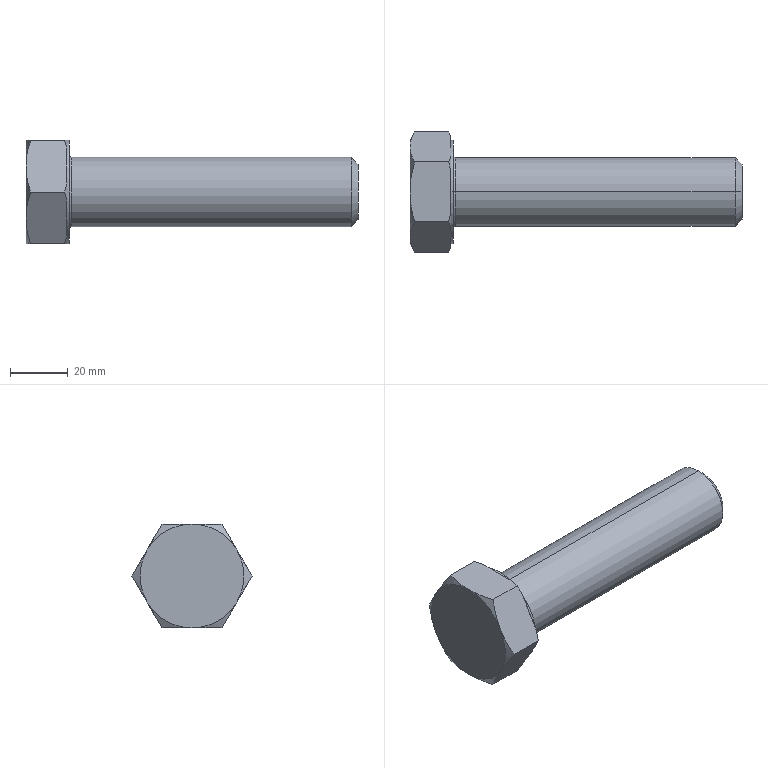Part | STEP file | GB/T 5780-2000 hex head bolt, grade C, M24×100 (3.6 grade) | 1 solid | 35 faces | box 115 x 41.569 x 36 mm | volume 61742 mm3 | plane 15 | cone 14 | cylinder 4 | torus 2 | commonest cylinder face diameters 24 x2 36 x2